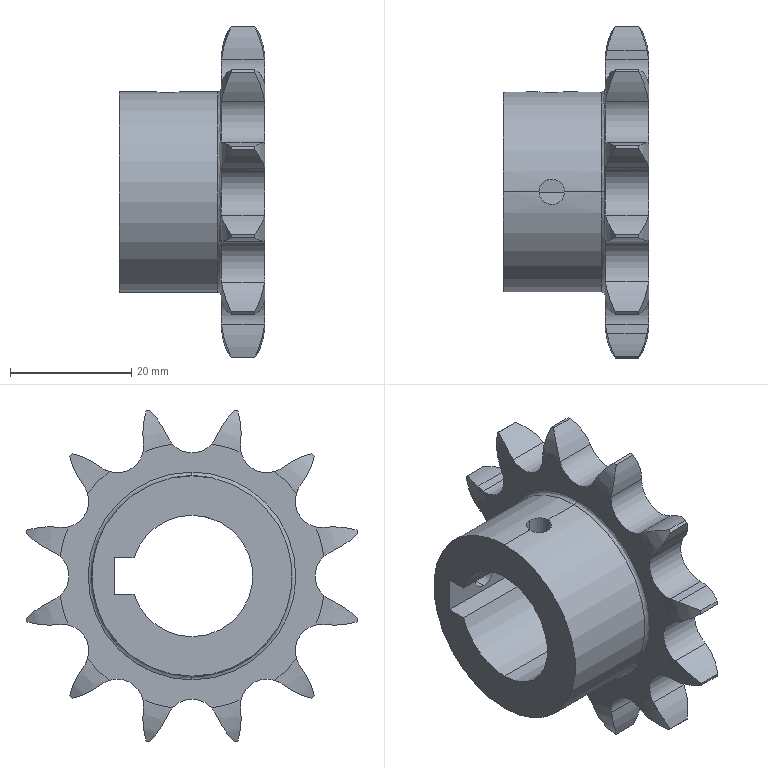Part | SolidWorks | features BaseBody 1, CirPattern 1, HoleWzd 1 | 1 solid | 96 faces | box 24.001 x 54.65 x 54.65 mm | volume 18054 mm3 | cylinder 64 | spline 26 | plane 6 | commonest cylinder face diameters 28.594 x26 8.595 x17 56.434 x12 4.2 x4 20 x3 33 x2